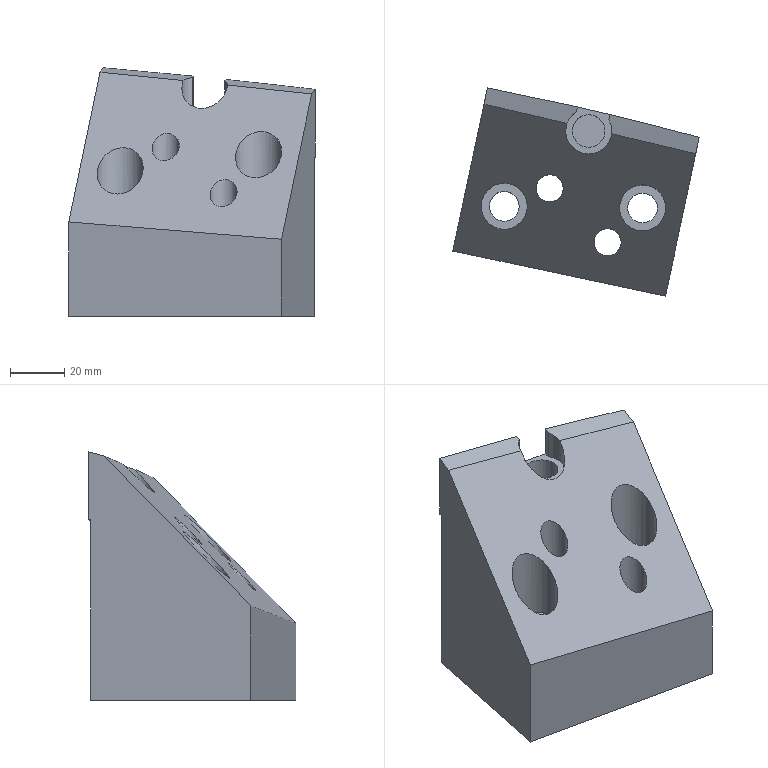Part | NX | features solid 2 | 1 solid | 24 faces | box 90.766 x 76.651 x 91.582 mm | volume 267587 mm3 | plane 11 | cylinder 8 | spline 5 | commonest cylinder face diameters 17 x3 10 x2 11 x2 12 x1
STEP:
#1=CARTESIAN_POINT('',(449.285,-481.788,-8.09));
#2=VERTEX_POINT('',#1);
#3=CARTESIAN_POINT('',(465.74,-485.634,-9.78));
#4=VERTEX_POINT('',#3);
#5=CARTESIAN_POINT('',(457.301,-484.613,-9.861));
#6=DIRECTION('',(-0.09165,-0.7023,0.706));
#7=DIRECTION('',(-0.09136,-0.7,-0.7082));
#8=AXIS2_PLACEMENT_3D('',#5,#6,#7);
#9=ELLIPSE('',#8,12.04,8.5);
#10=EDGE_CURVE('',#2,#4,#9,.T.);
#11=ORIENTED_EDGE('',*,*,#10,.F.);
#12=CARTESIAN_POINT('',(418.705,-474.755,-5.065));
#13=VERTEX_POINT('',#12);
#14=CARTESIAN_POINT('',(449.285,-481.788,-8.09));
#15=CARTESIAN_POINT('',(439.099,-479.42,-7.057));
#16=CARTESIAN_POINT('',(428.906,-477.075,-6.048));
#17=CARTESIAN_POINT('',(418.705,-474.755,-5.065));
#18=B_SPLINE_CURVE_WITH_KNOTS('',3,(#14,#15,#16,#17),.UNSPECIFIED.,.F.,.F.,(4,4),(0.,0.03152),.UNSPECIFIED.);
#19=EDGE_CURVE('',#2,#13,#18,.T.);
#20=ORIENTED_EDGE('',*,*,#19,.T.);
#21=CARTESIAN_POINT('',(407.237,-528.711,-60.225));
#22=VERTEX_POINT('',#21);
#23=CARTESIAN_POINT('',(413.497,-499.256,-30.113));
#24=DIRECTION('',(0.147,0.6917,0.7071));
#25=VECTOR('',#24,1000.);
#26=LINE('',#23,#25);
#27=EDGE_CURVE('',#13,#22,#26,.F.);
#28=ORIENTED_EDGE('',*,*,#27,.T.);
#29=CARTESIAN_POINT('',(485.592,-545.366,-66.621));
#30=VERTEX_POINT('',#29);
#31=CARTESIAN_POINT('',(402.563,-527.717,-59.844));
#32=DIRECTION('',(0.975,-0.2073,-0.07959));
#33=VECTOR('',#32,1000.);
#34=LINE('',#31,#33);
#35=EDGE_CURVE('',#22,#30,#34,.T.);
#36=ORIENTED_EDGE('',*,*,#35,.T.);
#37=CARTESIAN_POINT('',(496.726,-492.984,-13.069));
#38=VERTEX_POINT('',#37);
#39=CARTESIAN_POINT('',(492.518,-512.783,-33.311));
#40=DIRECTION('',(0.147,0.6917,0.7071));
#41=VECTOR('',#40,1000.);
#42=LINE('',#39,#41);
#43=EDGE_CURVE('',#30,#38,#42,.T.);
#44=ORIENTED_EDGE('',*,*,#43,.T.);
#45=CARTESIAN_POINT('',(496.726,-492.984,-13.069));
#46=CARTESIAN_POINT('',(486.404,-490.514,-11.952));
#47=CARTESIAN_POINT('',(476.076,-488.063,-10.855));
#48=CARTESIAN_POINT('',(465.74,-485.634,-9.78));
#49=B_SPLINE_CURVE_WITH_KNOTS('',3,(#45,#46,#47,#48),.UNSPECIFIED.,.F.,.F.,(4,4),(0.,0.03202),.UNSPECIFIED.);
#50=EDGE_CURVE('',#38,#4,#49,.T.);
#51=ORIENTED_EDGE('',*,*,#50,.T.);
#52=EDGE_LOOP('',(#11,#20,#28,#36,#44,#51));
#53=FACE_BOUND('',#52,.T.);
#54=CARTESIAN_POINT('',(464.904,-520.538,-44.609));
#55=VERTEX_POINT('',#54);
#56=CARTESIAN_POINT('',(464.257,-525.496,-49.625));
#57=DIRECTION('',(0.09165,0.7023,-0.706));
#58=DIRECTION('',(0.09136,0.7,0.7082));
#59=AXIS2_PLACEMENT_3D('',#56,#57,#58);
#60=ELLIPSE('',#59,7.082,5.);
#61=EDGE_CURVE('',#55,#55,#60,.F.);
#62=ORIENTED_EDGE('',*,*,#61,.F.);
#63=EDGE_LOOP('',(#62));
#64=FACE_BOUND('',#63,.T.);
#65=CARTESIAN_POINT('',(443.569,-500.668,-27.613));
#66=VERTEX_POINT('',#65);
#67=CARTESIAN_POINT('',(442.922,-505.626,-32.629));
#68=DIRECTION('',(0.09165,0.7023,-0.706));
#69=DIRECTION('',(0.09136,0.7,0.7082));
#70=AXIS2_PLACEMENT_3D('',#67,#68,#69);
#71=ELLIPSE('',#70,7.082,5.);
#72=EDGE_CURVE('',#66,#66,#71,.F.);
#73=ORIENTED_EDGE('',*,*,#72,.F.);
#74=EDGE_LOOP('',(#73));
#75=FACE_BOUND('',#74,.T.);
#76=CARTESIAN_POINT('',(478.257,-504.474,-26.897));
#77=VERTEX_POINT('',#76);
#78=CARTESIAN_POINT('',(477.158,-512.903,-35.424));
#79=DIRECTION('',(0.09165,0.7023,-0.706));
#80=DIRECTION('',(0.09136,0.7,0.7082));
#81=AXIS2_PLACEMENT_3D('',#78,#79,#80);
#82=ELLIPSE('',#81,12.04,8.5);
#83=EDGE_CURVE('',#77,#77,#82,.T.);
#84=ORIENTED_EDGE('',*,*,#83,.T.);
#85=EDGE_LOOP('',(#84));
#86=FACE_BOUND('',#85,.T.);
#87=CARTESIAN_POINT('',(427.271,-503.86,-32.905));
#88=VERTEX_POINT('',#87);
#89=CARTESIAN_POINT('',(426.171,-512.289,-41.432));
#90=DIRECTION('',(0.09165,0.7023,-0.706));
#91=DIRECTION('',(0.09136,0.7,0.7082));
#92=AXIS2_PLACEMENT_3D('',#89,#90,#91);
#93=ELLIPSE('',#92,12.04,8.5);
#94=EDGE_CURVE('',#88,#88,#93,.T.);
#95=ORIENTED_EDGE('',*,*,#94,.T.);
#96=EDGE_LOOP('',(#95));
#97=FACE_BOUND('',#96,.T.);
#98=CARTESIAN_POINT('',(496.103,-495.376,-15.53));
#99=DIRECTION('',(-0.09165,-0.7023,0.706));
#100=DIRECTION('',(0.,-0.709,-0.7052));
#101=AXIS2_PLACEMENT_3D('',#98,#99,#100);
#102=PLANE('',#101);
#103=ADVANCED_FACE('',(#53,#64,#75,#86,#97),#102,.T.);
#104=CARTESIAN_POINT('',(452.752,-477.433,-6.983));
#105=VERTEX_POINT('',#104);
#106=CARTESIAN_POINT('',(452.752,-477.433,-6.983));
#107=CARTESIAN_POINT('',(451.12,-478.467,-7.217));
#108=CARTESIAN_POINT('',(449.911,-480.01,-7.61));
#109=CARTESIAN_POINT('',(449.285,-481.788,-8.09));
#110=B_SPLINE_CURVE_WITH_KNOTS('',3,(#106,#107,#108,#109),.UNSPECIFIED.,.F.,.F.,(4,4),(0.,0.005753),.UNSPECIFIED.);
#111=EDGE_CURVE('',#105,#2,#110,.T.);
#112=ORIENTED_EDGE('',*,*,#111,.F.);
#113=CARTESIAN_POINT('',(453.112,-475.74,-6.517));
#114=VERTEX_POINT('',#113);
#115=CARTESIAN_POINT('',(452.752,-477.433,-6.983));
#116=CARTESIAN_POINT('',(452.872,-476.869,-6.827));
#117=CARTESIAN_POINT('',(452.992,-476.305,-6.672));
#118=CARTESIAN_POINT('',(453.112,-475.74,-6.517));
#119=B_SPLINE_CURVE_WITH_KNOTS('',3,(#115,#116,#117,#118),.UNSPECIFIED.,.F.,.F.,(4,4),(0.,0.001793),.UNSPECIFIED.);
#120=EDGE_CURVE('',#105,#114,#119,.T.);
#121=ORIENTED_EDGE('',*,*,#120,.T.);
#122=CARTESIAN_POINT('',(419.989,-468.715,-3.418));
#123=VERTEX_POINT('',#122);
#124=CARTESIAN_POINT('',(453.112,-475.74,-6.517));
#125=CARTESIAN_POINT('',(442.111,-473.238,-5.42));
#126=CARTESIAN_POINT('',(431.07,-470.895,-4.387));
#127=CARTESIAN_POINT('',(419.989,-468.715,-3.418));
#128=B_SPLINE_CURVE_WITH_KNOTS('',3,(#124,#125,#126,#127),.UNSPECIFIED.,.F.,.F.,(4,4),(0.,0.034),.UNSPECIFIED.);
#129=EDGE_CURVE('',#114,#123,#128,.T.);
#130=ORIENTED_EDGE('',*,*,#129,.T.);
#131=CARTESIAN_POINT('',(418.705,-474.755,-5.065));
#132=CARTESIAN_POINT('',(419.133,-472.742,-4.516));
#133=CARTESIAN_POINT('',(419.561,-470.729,-3.967));
#134=CARTESIAN_POINT('',(419.989,-468.715,-3.418));
#135=B_SPLINE_CURVE_WITH_KNOTS('',3,(#131,#132,#133,#134),.UNSPECIFIED.,.F.,.F.,(4,4),(0.,0.006391),.UNSPECIFIED.);
#136=EDGE_CURVE('',#13,#123,#135,.T.);
#137=ORIENTED_EDGE('',*,*,#136,.F.);
#138=ORIENTED_EDGE('',*,*,#19,.F.);
#139=EDGE_LOOP('',(#112,#121,#130,#137,#138));
#140=FACE_BOUND('',#139,.T.);
#141=CARTESIAN_POINT('',(419.708,-468.619,-3.382));
#142=CARTESIAN_POINT('',(418.384,-475.334,-5.216));
#143=CARTESIAN_POINT('',(430.965,-470.83,-4.365));
#144=CARTESIAN_POINT('',(429.58,-477.534,-6.199));
#145=CARTESIAN_POINT('',(442.182,-473.194,-5.41));
#146=CARTESIAN_POINT('',(440.732,-479.883,-7.244));
#147=CARTESIAN_POINT('',(453.348,-475.73,-6.522));
#148=CARTESIAN_POINT('',(451.829,-482.404,-8.356));
#149=B_SPLINE_SURFACE_WITH_KNOTS('',3,1,((#141,#142),(#143,#144),(#145,#146),(#147,#148)),.RULED_SURF.,.F.,.F.,.F.,(4,4),(2,2),(0.818,0.885),(0.2681,0.547),.PIECEWISE_BEZIER_KNOTS.);
#150=ADVANCED_FACE('',(#140),#149,.F.);
#151=CARTESIAN_POINT('',(464.757,-480.532,-8.293));
#152=VERTEX_POINT('',#151);
#153=CARTESIAN_POINT('',(465.74,-485.634,-9.78));
#154=CARTESIAN_POINT('',(465.953,-483.871,-9.287));
#155=CARTESIAN_POINT('',(465.612,-482.094,-8.768));
#156=CARTESIAN_POINT('',(464.757,-480.532,-8.293));
#157=B_SPLINE_CURVE_WITH_KNOTS('',3,(#153,#154,#155,#156),.UNSPECIFIED.,.F.,.F.,(4,4),(0.,0.00545),.UNSPECIFIED.);
#158=EDGE_CURVE('',#4,#152,#157,.T.);
#159=ORIENTED_EDGE('',*,*,#158,.F.);
#160=ORIENTED_EDGE('',*,*,#50,.F.);
#161=CARTESIAN_POINT('',(497.028,-491.564,-12.671));
#162=VERTEX_POINT('',#161);
#163=CARTESIAN_POINT('',(496.726,-492.984,-13.069));
#164=CARTESIAN_POINT('',(496.827,-492.511,-12.937));
#165=CARTESIAN_POINT('',(496.928,-492.037,-12.804));
#166=CARTESIAN_POINT('',(497.028,-491.564,-12.671));
#167=B_SPLINE_CURVE_WITH_KNOTS('',3,(#163,#164,#165,#166),.UNSPECIFIED.,.F.,.F.,(4,4),(0.009059,0.01057),.UNSPECIFIED.);
#168=EDGE_CURVE('',#38,#162,#167,.T.);
#169=ORIENTED_EDGE('',*,*,#168,.T.);
#170=CARTESIAN_POINT('',(498.002,-486.982,-11.386));
#171=VERTEX_POINT('',#170);
#172=CARTESIAN_POINT('',(497.028,-491.564,-12.671));
#173=CARTESIAN_POINT('',(497.353,-490.037,-12.243));
#174=CARTESIAN_POINT('',(497.678,-488.509,-11.814));
#175=CARTESIAN_POINT('',(498.002,-486.982,-11.386));
#176=B_SPLINE_CURVE_WITH_KNOTS('',3,(#172,#173,#174,#175),.UNSPECIFIED.,.F.,.F.,(4,4),(0.02436,0.02921),.UNSPECIFIED.);
#177=EDGE_CURVE('',#162,#171,#176,.T.);
#178=ORIENTED_EDGE('',*,*,#177,.T.);
#179=CARTESIAN_POINT('',(465.178,-478.555,-7.746));
#180=VERTEX_POINT('',#179);
#181=CARTESIAN_POINT('',(498.002,-486.982,-11.386));
#182=CARTESIAN_POINT('',(487.116,-483.988,-10.104));
#183=CARTESIAN_POINT('',(476.173,-481.185,-8.893));
#184=CARTESIAN_POINT('',(465.178,-478.555,-7.746));
#185=B_SPLINE_CURVE_WITH_KNOTS('',3,(#181,#182,#183,#184),.UNSPECIFIED.,.F.,.F.,(4,4),(0.,0.03408),.UNSPECIFIED.);
#186=EDGE_CURVE('',#171,#180,#185,.T.);
#187=ORIENTED_EDGE('',*,*,#186,.T.);
#188=CARTESIAN_POINT('',(465.178,-478.555,-7.746));
#189=CARTESIAN_POINT('',(465.038,-479.214,-7.929));
#190=CARTESIAN_POINT('',(464.898,-479.873,-8.111));
#191=CARTESIAN_POINT('',(464.757,-480.532,-8.293));
#192=B_SPLINE_CURVE_WITH_KNOTS('',3,(#188,#189,#190,#191),.UNSPECIFIED.,.F.,.F.,(4,4),(0.,0.002094),.UNSPECIFIED.);
#193=EDGE_CURVE('',#180,#152,#192,.T.);
#194=ORIENTED_EDGE('',*,*,#193,.T.);
#195=EDGE_LOOP('',(#159,#160,#169,#178,#187,#194));
#196=FACE_BOUND('',#195,.T.);
#197=CARTESIAN_POINT('',(464.991,-478.452,-7.71));
#198=CARTESIAN_POINT('',(463.397,-485.113,-9.546));
#199=CARTESIAN_POINT('',(476.244,-481.141,-8.882));
#200=CARTESIAN_POINT('',(474.577,-487.785,-10.718));
#201=CARTESIAN_POINT('',(487.44,-484.015,-10.124));
#202=CARTESIAN_POINT('',(485.695,-490.639,-11.96));
#203=CARTESIAN_POINT('',(498.568,-487.097,-11.441));
#204=CARTESIAN_POINT('',(496.741,-493.697,-13.276));
#205=B_SPLINE_SURFACE_WITH_KNOTS('',3,1,((#197,#198),(#199,#200),(#201,#202),(#203,#204)),.RULED_SURF.,.F.,.F.,.F.,(4,4),(2,2),(0.9084,0.9762),(0.2684,0.5476),.PIECEWISE_BEZIER_KNOTS.);
#206=ADVANCED_FACE('',(#196),#205,.F.);
#207=ORIENTED_EDGE('',*,*,#186,.F.);
#208=CARTESIAN_POINT('',(498.002,-486.982,-36.371));
#209=VERTEX_POINT('',#208);
#210=CARTESIAN_POINT('',(498.002,-486.982,-200.));
#211=DIRECTION('',(0.,0.,1.));
#212=VECTOR('',#211,1000.);
#213=LINE('',#210,#212);
#214=EDGE_CURVE('',#209,#171,#213,.T.);
#215=ORIENTED_EDGE('',*,*,#214,.F.);
#216=CARTESIAN_POINT('',(419.989,-468.715,-28.484));
#217=VERTEX_POINT('',#216);
#218=CARTESIAN_POINT('',(419.989,-468.715,-28.484));
#219=CARTESIAN_POINT('',(426.55,-470.006,-29.062));
#220=CARTESIAN_POINT('',(439.644,-472.702,-30.264));
#221=CARTESIAN_POINT('',(455.941,-476.352,-31.88));
#222=CARTESIAN_POINT('',(468.932,-479.444,-33.243));
#223=CARTESIAN_POINT('',(477.029,-481.453,-34.126));
#224=CARTESIAN_POINT('',(483.493,-483.107,-34.848));
#225=CARTESIAN_POINT('',(488.333,-484.372,-35.404));
#226=CARTESIAN_POINT('',(493.168,-485.661,-35.946));
#227=CARTESIAN_POINT('',(496.381,-486.536,-36.371));
#228=CARTESIAN_POINT('',(498.002,-486.982,-36.371));
#229=B_SPLINE_CURVE_WITH_KNOTS('',3,(#218,#219,#220,#221,#222,#223,#224,#225,#226,#227,#228),.UNSPECIFIED.,.F.,.F.,(4,1,1,1,1,1,1,1,4),(0.,0.02013,0.04027,0.05033,0.0604,0.06544,0.07047,0.0755,0.08054),.UNSPECIFIED.);
#230=EDGE_CURVE('',#217,#209,#229,.T.);
#231=ORIENTED_EDGE('',*,*,#230,.F.);
#232=CARTESIAN_POINT('',(419.989,-468.715,-200.));
#233=DIRECTION('',(0.,0.,1.));
#234=VECTOR('',#233,1000.);
#235=LINE('',#232,#234);
#236=EDGE_CURVE('',#217,#123,#235,.T.);
#237=ORIENTED_EDGE('',*,*,#236,.T.);
#238=ORIENTED_EDGE('',*,*,#129,.F.);
#239=CARTESIAN_POINT('',(453.112,-475.74,-19.));
#240=VERTEX_POINT('',#239);
#241=CARTESIAN_POINT('',(453.112,-475.74,-12.795));
#242=DIRECTION('',(0.,0.,1.));
#243=VECTOR('',#242,1000.);
#244=LINE('',#241,#243);
#245=EDGE_CURVE('',#240,#114,#244,.T.);
#246=ORIENTED_EDGE('',*,*,#245,.F.);
#247=CARTESIAN_POINT('',(465.178,-478.555,-19.));
#248=VERTEX_POINT('',#247);
#249=CARTESIAN_POINT('',(498.002,-486.982,-19.));
#250=CARTESIAN_POINT('',(487.75,-484.162,-19.));
#251=CARTESIAN_POINT('',(472.124,-480.143,-19.));
#252=CARTESIAN_POINT('',(446.106,-474.081,-19.));
#253=CARTESIAN_POINT('',(430.372,-470.758,-19.));
#254=CARTESIAN_POINT('',(419.989,-468.715,-19.));
#255=B_SPLINE_CURVE_WITH_KNOTS('',3,(#249,#250,#251,#252,#253,#254),.UNSPECIFIED.,.F.,.F.,(4,1,1,4),(0.,0.398,0.6039,1.),.UNSPECIFIED.);
#256=EDGE_CURVE('',#240,#248,#255,.F.);
#257=ORIENTED_EDGE('',*,*,#256,.T.);
#258=CARTESIAN_POINT('',(465.178,-478.555,-13.311));
#259=DIRECTION('',(0.,0.,1.));
#260=VECTOR('',#259,1000.);
#261=LINE('',#258,#260);
#262=EDGE_CURVE('',#180,#248,#261,.F.);
#263=ORIENTED_EDGE('',*,*,#262,.F.);
#264=EDGE_LOOP('',(#207,#215,#231,#237,#238,#246,#257,#263));
#265=FACE_BOUND('',#264,.T.);
#266=CARTESIAN_POINT('',(498.002,-486.982,-36.569));
#267=CARTESIAN_POINT('',(498.002,-486.982,-3.22));
#268=CARTESIAN_POINT('',(472.245,-479.897,-36.569));
#269=CARTESIAN_POINT('',(472.245,-479.897,-3.22));
#270=CARTESIAN_POINT('',(446.201,-473.872,-36.569));
#271=CARTESIAN_POINT('',(446.201,-473.872,-3.22));
#272=CARTESIAN_POINT('',(419.989,-468.715,-36.569));
#273=CARTESIAN_POINT('',(419.989,-468.715,-3.22));
#274=B_SPLINE_SURFACE_WITH_KNOTS('',3,1,((#266,#267),(#268,#269),(#270,#271),(#272,#273)),.SURF_OF_LINEAR_EXTRUSION.,.F.,.F.,.F.,(4,4),(2,2),(0.,1.),(0.,1.),.PIECEWISE_BEZIER_KNOTS.);
#275=ADVANCED_FACE('',(#265),#274,.T.);
#276=CARTESIAN_POINT('',(431.671,-512.289,-95.));
#277=VERTEX_POINT('',#276);
#278=CARTESIAN_POINT('',(426.171,-512.289,-95.));
#279=DIRECTION('',(0.,0.,1.));
#280=DIRECTION('',(1.,0.,0.));
#281=AXIS2_PLACEMENT_3D('',#278,#279,#280);
#282=CIRCLE('',#281,5.5);
#283=EDGE_CURVE('',#277,#277,#282,.T.);
#284=ORIENTED_EDGE('',*,*,#283,.T.);
#285=EDGE_LOOP('',(#284));
#286=FACE_BOUND('',#285,.T.);
#287=CARTESIAN_POINT('',(482.658,-512.903,-95.));
#288=VERTEX_POINT('',#287);
#289=CARTESIAN_POINT('',(477.158,-512.903,-95.));
#290=DIRECTION('',(0.,0.,1.));
#291=DIRECTION('',(1.,0.,0.));
#292=AXIS2_PLACEMENT_3D('',#289,#290,#291);
#293=CIRCLE('',#292,5.5);
#294=EDGE_CURVE('',#288,#288,#293,.T.);
#295=ORIENTED_EDGE('',*,*,#294,.T.);
#296=EDGE_LOOP('',(#295));
#297=FACE_BOUND('',#296,.T.);
#298=CARTESIAN_POINT('',(447.922,-505.626,-95.));
#299=VERTEX_POINT('',#298);
#300=CARTESIAN_POINT('',(442.922,-505.626,-95.));
#301=DIRECTION('',(0.,0.,1.));
#302=DIRECTION('',(1.,0.,0.));
#303=AXIS2_PLACEMENT_3D('',#300,#301,#302);
#304=CIRCLE('',#303,5.);
#305=EDGE_CURVE('',#299,#299,#304,.F.);
#306=ORIENTED_EDGE('',*,*,#305,.F.);
#307=EDGE_LOOP('',(#306));
#308=FACE_BOUND('',#307,.T.);
#309=CARTESIAN_POINT('',(419.781,-469.693,-95.));
#310=VERTEX_POINT('',#309);
#311=CARTESIAN_POINT('',(497.794,-487.962,-95.));
#312=VERTEX_POINT('',#311);
#313=CARTESIAN_POINT('',(419.781,-469.693,-95.));
#314=CARTESIAN_POINT('',(445.994,-474.85,-95.));
#315=CARTESIAN_POINT('',(472.036,-480.876,-95.));
#316=CARTESIAN_POINT('',(497.794,-487.962,-95.));
#317=B_SPLINE_CURVE_WITH_KNOTS('',3,(#313,#314,#315,#316),.UNSPECIFIED.,.F.,.F.,(4,4),(0.124,0.2041),.UNSPECIFIED.);
#318=EDGE_CURVE('',#310,#312,#317,.T.);
#319=ORIENTED_EDGE('',*,*,#318,.T.);
#320=CARTESIAN_POINT('',(485.592,-545.366,-95.));
#321=VERTEX_POINT('',#320);
#322=CARTESIAN_POINT('',(485.592,-545.366,-95.));
#323=DIRECTION('',(-0.2079,-0.9781,0.));
#324=VECTOR('',#323,1000.);
#325=LINE('',#322,#324);
#326=EDGE_CURVE('',#321,#312,#325,.F.);
#327=ORIENTED_EDGE('',*,*,#326,.F.);
#328=CARTESIAN_POINT('',(407.237,-528.711,-95.));
#329=VERTEX_POINT('',#328);
#330=CARTESIAN_POINT('',(407.237,-528.711,-95.));
#331=DIRECTION('',(-0.9781,0.2079,0.));
#332=VECTOR('',#331,1000.);
#333=LINE('',#330,#332);
#334=EDGE_CURVE('',#329,#321,#333,.F.);
#335=ORIENTED_EDGE('',*,*,#334,.F.);
#336=CARTESIAN_POINT('',(419.97,-468.803,-95.));
#337=DIRECTION('',(0.2079,0.9781,0.));
#338=VECTOR('',#337,1000.);
#339=LINE('',#336,#338);
#340=EDGE_CURVE('',#329,#310,#339,.T.);
#341=ORIENTED_EDGE('',*,*,#340,.T.);
#342=EDGE_LOOP('',(#319,#327,#335,#341));
#343=FACE_BOUND('',#342,.T.);
#344=CARTESIAN_POINT('',(469.257,-525.496,-95.));
#345=VERTEX_POINT('',#344);
#346=CARTESIAN_POINT('',(464.257,-525.496,-95.));
#347=DIRECTION('',(0.,0.,1.));
#348=DIRECTION('',(1.,0.,0.));
#349=AXIS2_PLACEMENT_3D('',#346,#347,#348);
#350=CIRCLE('',#349,5.);
#351=EDGE_CURVE('',#345,#345,#350,.F.);
#352=ORIENTED_EDGE('',*,*,#351,.F.);
#353=EDGE_LOOP('',(#352));
#354=FACE_BOUND('',#353,.T.);
#355=CARTESIAN_POINT('',(459.163,-477.134,-95.));
#356=DIRECTION('',(0.,0.,1.));
#357=DIRECTION('',(-1.,0.,0.));
#358=AXIS2_PLACEMENT_3D('',#355,#356,#357);
#359=PLANE('',#358);
#360=ADVANCED_FACE('',(#286,#297,#308,#343,#354),#359,.F.);
#361=CARTESIAN_POINT('',(407.237,-528.711,0.));
#362=DIRECTION('',(0.,0.,1.));
#363=VECTOR('',#362,1000.);
#364=LINE('',#361,#363);
#365=EDGE_CURVE('',#329,#22,#364,.T.);
#366=ORIENTED_EDGE('',*,*,#365,.F.);
#367=ORIENTED_EDGE('',*,*,#334,.T.);
#368=CARTESIAN_POINT('',(485.592,-545.366,0.));
#369=DIRECTION('',(0.,0.,1.));
#370=VECTOR('',#369,1000.);
#371=LINE('',#368,#370);
#372=EDGE_CURVE('',#321,#30,#371,.T.);
#373=ORIENTED_EDGE('',*,*,#372,.T.);
#374=ORIENTED_EDGE('',*,*,#35,.F.);
#375=EDGE_LOOP('',(#366,#367,#373,#374));
#376=FACE_BOUND('',#375,.T.);
#377=CARTESIAN_POINT('',(407.237,-528.711,0.));
#378=DIRECTION('',(-0.2079,-0.9781,0.));
#379=DIRECTION('',(0.9781,-0.2079,0.));
#380=AXIS2_PLACEMENT_3D('',#377,#378,#379);
#381=PLANE('',#380);
#382=ADVANCED_FACE('',(#376),#381,.T.);
#383=ORIENTED_EDGE('',*,*,#340,.F.);
#384=ORIENTED_EDGE('',*,*,#365,.T.);
#385=ORIENTED_EDGE('',*,*,#27,.F.);
#386=ORIENTED_EDGE('',*,*,#136,.T.);
#387=ORIENTED_EDGE('',*,*,#236,.F.);
#388=CARTESIAN_POINT('',(419.781,-469.693,-28.483));
#389=VERTEX_POINT('',#388);
#390=CARTESIAN_POINT('',(419.989,-468.715,-28.484));
#391=CARTESIAN_POINT('',(419.92,-469.041,-28.483));
#392=CARTESIAN_POINT('',(419.85,-469.367,-28.483));
#393=CARTESIAN_POINT('',(419.781,-469.693,-28.483));
#394=B_SPLINE_CURVE_WITH_KNOTS('',3,(#390,#391,#392,#393),.UNSPECIFIED.,.F.,.F.,(4,4),(0.,0.001),.UNSPECIFIED.);
#395=EDGE_CURVE('',#217,#389,#394,.T.);
#396=ORIENTED_EDGE('',*,*,#395,.T.);
#397=CARTESIAN_POINT('',(419.781,-469.693,-78.483));
#398=DIRECTION('',(0.,0.,-1.));
#399=VECTOR('',#398,1000.);
#400=LINE('',#397,#399);
#401=EDGE_CURVE('',#310,#389,#400,.F.);
#402=ORIENTED_EDGE('',*,*,#401,.F.);
#403=EDGE_LOOP('',(#383,#384,#385,#386,#387,#396,#402));
#404=FACE_BOUND('',#403,.T.);
#405=CARTESIAN_POINT('',(407.237,-528.711,0.));
#406=DIRECTION('',(0.9781,-0.2079,0.));
#407=DIRECTION('',(0.2079,0.9781,0.));
#408=AXIS2_PLACEMENT_3D('',#405,#406,#407);
#409=PLANE('',#408);
#410=ADVANCED_FACE('',(#404),#409,.F.);
#411=ORIENTED_EDGE('',*,*,#43,.F.);
#412=ORIENTED_EDGE('',*,*,#372,.F.);
#413=ORIENTED_EDGE('',*,*,#326,.T.);
#414=CARTESIAN_POINT('',(497.794,-487.962,-36.371));
#415=VERTEX_POINT('',#414);
#416=CARTESIAN_POINT('',(497.794,-487.962,-86.371));
#417=DIRECTION('',(0.,0.,-1.));
#418=VECTOR('',#417,1000.);
#419=LINE('',#416,#418);
#420=EDGE_CURVE('',#312,#415,#419,.F.);
#421=ORIENTED_EDGE('',*,*,#420,.T.);
#422=CARTESIAN_POINT('',(498.002,-486.982,-36.371));
#423=CARTESIAN_POINT('',(497.933,-487.309,-36.371));
#424=CARTESIAN_POINT('',(497.863,-487.635,-36.371));
#425=CARTESIAN_POINT('',(497.794,-487.962,-36.371));
#426=B_SPLINE_CURVE_WITH_KNOTS('',3,(#422,#423,#424,#425),.UNSPECIFIED.,.F.,.F.,(4,4),(0.,0.001002),.UNSPECIFIED.);
#427=EDGE_CURVE('',#209,#415,#426,.T.);
#428=ORIENTED_EDGE('',*,*,#427,.F.);
#429=ORIENTED_EDGE('',*,*,#214,.T.);
#430=ORIENTED_EDGE('',*,*,#177,.F.);
#431=ORIENTED_EDGE('',*,*,#168,.F.);
#432=EDGE_LOOP('',(#411,#412,#413,#421,#428,#429,#430,#431));
#433=FACE_BOUND('',#432,.T.);
#434=CARTESIAN_POINT('',(485.592,-545.366,0.));
#435=DIRECTION('',(0.9781,-0.2079,0.));
#436=DIRECTION('',(0.2079,0.9781,0.));
#437=AXIS2_PLACEMENT_3D('',#434,#435,#436);
#438=PLANE('',#437);
#439=ADVANCED_FACE('',(#433),#438,.T.);
#440=ORIENTED_EDGE('',*,*,#395,.F.);
#441=ORIENTED_EDGE('',*,*,#230,.T.);
#442=ORIENTED_EDGE('',*,*,#427,.T.);
#443=CARTESIAN_POINT('',(497.794,-487.962,-36.371));
#444=CARTESIAN_POINT('',(496.173,-487.516,-36.371));
#445=CARTESIAN_POINT('',(492.959,-486.641,-35.955));
#446=CARTESIAN_POINT('',(488.125,-485.35,-35.409));
#447=CARTESIAN_POINT('',(483.286,-484.085,-34.853));
#448=CARTESIAN_POINT('',(476.823,-482.428,-34.13));
#449=CARTESIAN_POINT('',(468.727,-480.416,-33.247));
#450=CARTESIAN_POINT('',(455.737,-477.32,-31.882));
#451=CARTESIAN_POINT('',(439.439,-473.674,-30.264));
#452=CARTESIAN_POINT('',(426.342,-470.984,-29.062));
#453=CARTESIAN_POINT('',(419.781,-469.693,-28.483));
#454=B_SPLINE_CURVE_WITH_KNOTS('',3,(#443,#444,#445,#446,#447,#448,#449,#450,#451,#452,#453),.UNSPECIFIED.,.F.,.F.,(4,1,1,1,1,1,1,1,4),(-0.0007328,0.06182,0.1244,0.1869,0.2495,0.3746,0.4997,0.75,1.),.UNSPECIFIED.);
#455=EDGE_CURVE('',#415,#389,#454,.T.);
#456=ORIENTED_EDGE('',*,*,#455,.T.);
#457=EDGE_LOOP('',(#440,#441,#442,#456));
#458=FACE_BOUND('',#457,.T.);
#459=CARTESIAN_POINT('',(498.528,-487.121,-36.371));
#460=CARTESIAN_POINT('',(498.353,-487.073,-36.371));
#461=CARTESIAN_POINT('',(498.179,-487.025,-36.371));
#462=CARTESIAN_POINT('',(498.004,-486.976,-36.371));
#463=CARTESIAN_POINT('',(496.383,-486.53,-36.371));
#464=CARTESIAN_POINT('',(494.776,-486.093,-36.149));
#465=CARTESIAN_POINT('',(491.557,-485.225,-35.775));
#466=CARTESIAN_POINT('',(489.946,-484.795,-35.587));
#467=CARTESIAN_POINT('',(485.109,-483.517,-35.031));
#468=CARTESIAN_POINT('',(481.88,-482.681,-34.666));
#469=CARTESIAN_POINT('',(472.178,-480.221,-33.59));
#470=CARTESIAN_POINT('',(465.691,-478.643,-32.897));
#471=CARTESIAN_POINT('',(446.182,-474.088,-30.887));
#472=CARTESIAN_POINT('',(433.111,-471.291,-29.641));
#473=CARTESIAN_POINT('',(419.99,-468.709,-28.484));
#474=CARTESIAN_POINT('',(419.828,-468.677,-28.47));
#475=CARTESIAN_POINT('',(419.665,-468.645,-28.455));
#476=CARTESIAN_POINT('',(419.502,-468.613,-28.441));
#477=CARTESIAN_POINT('',(498.261,-488.091,-36.371));
#478=CARTESIAN_POINT('',(498.086,-488.042,-36.371));
#479=CARTESIAN_POINT('',(497.912,-487.994,-36.371));
#480=CARTESIAN_POINT('',(497.737,-487.946,-36.371));
#481=CARTESIAN_POINT('',(496.117,-487.501,-36.371));
#482=CARTESIAN_POINT('',(494.513,-487.064,-36.149));
#483=CARTESIAN_POINT('',(491.296,-486.197,-35.775));
#484=CARTESIAN_POINT('',(489.687,-485.767,-35.587));
#485=CARTESIAN_POINT('',(484.855,-484.491,-35.031));
#486=CARTESIAN_POINT('',(481.629,-483.656,-34.666));
#487=CARTESIAN_POINT('',(471.937,-481.197,-33.59));
#488=CARTESIAN_POINT('',(465.456,-479.621,-32.897));
#489=CARTESIAN_POINT('',(445.966,-475.071,-30.887));
#490=CARTESIAN_POINT('',(432.906,-472.276,-29.641));
#491=CARTESIAN_POINT('',(419.796,-469.696,-28.484));
#492=CARTESIAN_POINT('',(419.634,-469.664,-28.47));
#493=CARTESIAN_POINT('',(419.471,-469.632,-28.455));
#494=CARTESIAN_POINT('',(419.309,-469.6,-28.441));
#495=B_SPLINE_SURFACE_WITH_KNOTS('',1,3,((#459,#460,#461,#462,#463,#464,#465,#466,#467,#468,#469,#470,#471,#472,#473,#474,#475,#476),(#477,#478,#479,#480,#481,#482,#483,#484,#485,#486,#487,#488,#489,#490,#491,#492,#493,#494)),.RULED_SURF.,.F.,.F.,.F.,(2,2),(4,3,2,2,2,2,3,4),(0.497,1.),(-0.006738,0.,0.0625,0.125,0.25,0.5,1.,1.006),.UNSPECIFIED.);
#496=ADVANCED_FACE('',(#458),#495,.T.);
#497=ORIENTED_EDGE('',*,*,#318,.F.);
#498=ORIENTED_EDGE('',*,*,#401,.T.);
#499=ORIENTED_EDGE('',*,*,#455,.F.);
#500=ORIENTED_EDGE('',*,*,#420,.F.);
#501=EDGE_LOOP('',(#497,#498,#499,#500));
#502=FACE_BOUND('',#501,.T.);
#503=CARTESIAN_POINT('',(497.794,-487.962,-36.371));
#504=CARTESIAN_POINT('',(497.794,-487.962,-103.287));
#505=CARTESIAN_POINT('',(496.175,-487.517,-36.371));
#506=CARTESIAN_POINT('',(496.175,-487.517,-103.287));
#507=CARTESIAN_POINT('',(492.958,-486.64,-35.955));
#508=CARTESIAN_POINT('',(492.958,-486.64,-102.872));
#509=CARTESIAN_POINT('',(488.126,-485.35,-35.409));
#510=CARTESIAN_POINT('',(488.126,-485.35,-102.326));
#511=CARTESIAN_POINT('',(483.286,-484.085,-34.853));
#512=CARTESIAN_POINT('',(483.286,-484.085,-101.769));
#513=CARTESIAN_POINT('',(476.823,-482.428,-34.13));
#514=CARTESIAN_POINT('',(476.823,-482.428,-101.046));
#515=CARTESIAN_POINT('',(468.726,-480.416,-33.247));
#516=CARTESIAN_POINT('',(468.726,-480.416,-100.163));
#517=CARTESIAN_POINT('',(455.738,-477.32,-31.882));
#518=CARTESIAN_POINT('',(455.738,-477.32,-98.799));
#519=CARTESIAN_POINT('',(439.437,-473.673,-30.264));
#520=CARTESIAN_POINT('',(439.437,-473.673,-97.181));
#521=CARTESIAN_POINT('',(426.348,-470.985,-29.062));
#522=CARTESIAN_POINT('',(426.348,-470.985,-95.978));
#523=CARTESIAN_POINT('',(419.781,-469.693,-28.483));
#524=CARTESIAN_POINT('',(419.781,-469.693,-95.399));
#525=B_SPLINE_SURFACE_WITH_KNOTS('',3,1,((#503,#504),(#505,#506),(#507,#508),(#509,#510),(#511,#512),(#513,#514),(#515,#516),(#517,#518),(#519,#520),(#521,#522),(#523,#524)),.SURF_OF_LINEAR_EXTRUSION.,.F.,.F.,.F.,(4,1,1,1,1,1,1,1,4),(2,2),(-0.0007336,0.06182,0.1244,0.1869,0.2495,0.3746,0.4997,0.75,1.),(0.,1.),.UNSPECIFIED.);
#526=ADVANCED_FACE('',(#502),#525,.F.);
#527=ORIENTED_EDGE('',*,*,#305,.T.);
#528=EDGE_LOOP('',(#527));
#529=FACE_BOUND('',#528,.T.);
#530=ORIENTED_EDGE('',*,*,#72,.T.);
#531=EDGE_LOOP('',(#530));
#532=FACE_BOUND('',#531,.T.);
#533=CARTESIAN_POINT('',(442.922,-505.626,-200.));
#534=DIRECTION('',(0.,0.,1.));
#535=DIRECTION('',(-1.,0.,0.));
#536=AXIS2_PLACEMENT_3D('',#533,#534,#535);
#537=CYLINDRICAL_SURFACE('',#536,5.);
#538=ADVANCED_FACE('',(#529,#532),#537,.F.);
#539=ORIENTED_EDGE('',*,*,#351,.T.);
#540=EDGE_LOOP('',(#539));
#541=FACE_BOUND('',#540,.T.);
#542=ORIENTED_EDGE('',*,*,#61,.T.);
#543=EDGE_LOOP('',(#542));
#544=FACE_BOUND('',#543,.T.);
#545=CARTESIAN_POINT('',(464.257,-525.496,-200.));
#546=DIRECTION('',(0.,0.,1.));
#547=DIRECTION('',(-1.,0.,0.));
#548=AXIS2_PLACEMENT_3D('',#545,#546,#547);
#549=CYLINDRICAL_SURFACE('',#548,5.);
#550=ADVANCED_FACE('',(#541,#544),#549,.F.);
#551=ORIENTED_EDGE('',*,*,#294,.F.);
#552=EDGE_LOOP('',(#551));
#553=FACE_BOUND('',#552,.T.);
#554=CARTESIAN_POINT('',(482.658,-512.903,-60.));
#555=VERTEX_POINT('',#554);
#556=CARTESIAN_POINT('',(477.158,-512.903,-60.));
#557=DIRECTION('',(0.,0.,1.));
#558=DIRECTION('',(1.,0.,0.));
#559=AXIS2_PLACEMENT_3D('',#556,#557,#558);
#560=CIRCLE('',#559,5.5);
#561=EDGE_CURVE('',#555,#555,#560,.F.);
#562=ORIENTED_EDGE('',*,*,#561,.F.);
#563=EDGE_LOOP('',(#562));
#564=FACE_BOUND('',#563,.T.);
#565=CARTESIAN_POINT('',(477.158,-512.903,-105.));
#566=DIRECTION('',(0.,0.,1.));
#567=DIRECTION('',(-1.,0.,0.));
#568=AXIS2_PLACEMENT_3D('',#565,#566,#567);
#569=CYLINDRICAL_SURFACE('',#568,5.5);
#570=ADVANCED_FACE('',(#553,#564),#569,.F.);
#571=ORIENTED_EDGE('',*,*,#561,.T.);
#572=EDGE_LOOP('',(#571));
#573=FACE_BOUND('',#572,.T.);
#574=CARTESIAN_POINT('',(485.658,-512.903,-60.));
#575=VERTEX_POINT('',#574);
#576=CARTESIAN_POINT('',(477.158,-512.903,-60.));
#577=DIRECTION('',(0.,0.,1.));
#578=DIRECTION('',(1.,0.,0.));
#579=AXIS2_PLACEMENT_3D('',#576,#577,#578);
#580=CIRCLE('',#579,8.5);
#581=EDGE_CURVE('',#575,#575,#580,.F.);
#582=ORIENTED_EDGE('',*,*,#581,.F.);
#583=EDGE_LOOP('',(#582));
#584=FACE_BOUND('',#583,.T.);
#585=CARTESIAN_POINT('',(477.158,-512.903,-60.));
#586=DIRECTION('',(0.,0.,-1.));
#587=DIRECTION('',(1.,0.,0.));
#588=AXIS2_PLACEMENT_3D('',#585,#586,#587);
#589=PLANE('',#588);
#590=ADVANCED_FACE('',(#573,#584),#589,.F.);
#591=ORIENTED_EDGE('',*,*,#83,.F.);
#592=EDGE_LOOP('',(#591));
#593=FACE_BOUND('',#592,.T.);
#594=ORIENTED_EDGE('',*,*,#581,.T.);
#595=EDGE_LOOP('',(#594));
#596=FACE_BOUND('',#595,.T.);
#597=CARTESIAN_POINT('',(477.158,-512.903,-65.));
#598=DIRECTION('',(0.,0.,1.));
#599=DIRECTION('',(-1.,0.,0.));
#600=AXIS2_PLACEMENT_3D('',#597,#598,#599);
#601=CYLINDRICAL_SURFACE('',#600,8.5);
#602=ADVANCED_FACE('',(#593,#596),#601,.F.);
#603=ORIENTED_EDGE('',*,*,#283,.F.);
#604=EDGE_LOOP('',(#603));
#605=FACE_BOUND('',#604,.T.);
#606=CARTESIAN_POINT('',(431.671,-512.289,-60.));
#607=VERTEX_POINT('',#606);
#608=CARTESIAN_POINT('',(426.171,-512.289,-60.));
#609=DIRECTION('',(0.,0.,1.));
#610=DIRECTION('',(1.,0.,0.));
#611=AXIS2_PLACEMENT_3D('',#608,#609,#610);
#612=CIRCLE('',#611,5.5);
#613=EDGE_CURVE('',#607,#607,#612,.F.);
#614=ORIENTED_EDGE('',*,*,#613,.F.);
#615=EDGE_LOOP('',(#614));
#616=FACE_BOUND('',#615,.T.);
#617=CARTESIAN_POINT('',(426.171,-512.289,-105.));
#618=DIRECTION('',(0.,0.,1.));
#619=DIRECTION('',(-1.,0.,0.));
#620=AXIS2_PLACEMENT_3D('',#617,#618,#619);
#621=CYLINDRICAL_SURFACE('',#620,5.5);
#622=ADVANCED_FACE('',(#605,#616),#621,.F.);
#623=ORIENTED_EDGE('',*,*,#613,.T.);
#624=EDGE_LOOP('',(#623));
#625=FACE_BOUND('',#624,.T.);
#626=CARTESIAN_POINT('',(434.671,-512.289,-60.));
#627=VERTEX_POINT('',#626);
#628=CARTESIAN_POINT('',(426.171,-512.289,-60.));
#629=DIRECTION('',(0.,0.,1.));
#630=DIRECTION('',(1.,0.,0.));
#631=AXIS2_PLACEMENT_3D('',#628,#629,#630);
#632=CIRCLE('',#631,8.5);
#633=EDGE_CURVE('',#627,#627,#632,.F.);
#634=ORIENTED_EDGE('',*,*,#633,.F.);
#635=EDGE_LOOP('',(#634));
#636=FACE_BOUND('',#635,.T.);
#637=CARTESIAN_POINT('',(426.171,-512.289,-60.));
#638=DIRECTION('',(0.,0.,-1.));
#639=DIRECTION('',(1.,0.,0.));
#640=AXIS2_PLACEMENT_3D('',#637,#638,#639);
#641=PLANE('',#640);
#642=ADVANCED_FACE('',(#625,#636),#641,.F.);
#643=ORIENTED_EDGE('',*,*,#94,.F.);
#644=EDGE_LOOP('',(#643));
#645=FACE_BOUND('',#644,.T.);
#646=ORIENTED_EDGE('',*,*,#633,.T.);
#647=EDGE_LOOP('',(#646));
#648=FACE_BOUND('',#647,.T.);
#649=CARTESIAN_POINT('',(426.171,-512.289,-65.));
#650=DIRECTION('',(0.,0.,1.));
#651=DIRECTION('',(-1.,0.,0.));
#652=AXIS2_PLACEMENT_3D('',#649,#650,#651);
#653=CYLINDRICAL_SURFACE('',#652,8.5);
#654=ADVANCED_FACE('',(#645,#648),#653,.F.);
#655=CARTESIAN_POINT('',(463.301,-484.613,-19.));
#656=VERTEX_POINT('',#655);
#657=CARTESIAN_POINT('',(457.301,-484.613,-19.));
#658=DIRECTION('',(0.,0.,1.));
#659=DIRECTION('',(1.,0.,0.));
#660=AXIS2_PLACEMENT_3D('',#657,#658,#659);
#661=CIRCLE('',#660,6.);
#662=EDGE_CURVE('',#656,#656,#661,.T.);
#663=ORIENTED_EDGE('',*,*,#662,.F.);
#664=EDGE_LOOP('',(#663));
#665=FACE_BOUND('',#664,.T.);
#666=CARTESIAN_POINT('',(452.752,-477.433,-19.));
#667=VERTEX_POINT('',#666);
#668=CARTESIAN_POINT('',(451.465,-483.489,-19.));
#669=DIRECTION('',(0.2079,0.9781,0.));
#670=VECTOR('',#669,1000.);
#671=LINE('',#668,#670);
#672=EDGE_CURVE('',#240,#667,#671,.F.);
#673=ORIENTED_EDGE('',*,*,#672,.T.);
#674=CARTESIAN_POINT('',(464.757,-480.532,-19.));
#675=VERTEX_POINT('',#674);
#676=CARTESIAN_POINT('',(457.301,-484.613,-19.));
#677=DIRECTION('',(0.,0.,-1.));
#678=DIRECTION('',(-1.,0.,0.));
#679=AXIS2_PLACEMENT_3D('',#676,#677,#678);
#680=CIRCLE('',#679,8.5);
#681=EDGE_CURVE('',#675,#667,#680,.T.);
#682=ORIENTED_EDGE('',*,*,#681,.F.);
#683=CARTESIAN_POINT('',(465.202,-478.442,-19.));
#684=DIRECTION('',(0.2079,0.9781,0.));
#685=VECTOR('',#684,1000.);
#686=LINE('',#683,#685);
#687=EDGE_CURVE('',#248,#675,#686,.F.);
#688=ORIENTED_EDGE('',*,*,#687,.F.);
#689=ORIENTED_EDGE('',*,*,#256,.F.);
#690=EDGE_LOOP('',(#673,#682,#688,#689));
#691=FACE_BOUND('',#690,.T.);
#692=CARTESIAN_POINT('',(457.177,-484.703,-19.));
#693=DIRECTION('',(0.,0.,1.));
#694=DIRECTION('',(-1.,0.,0.));
#695=AXIS2_PLACEMENT_3D('',#692,#693,#694);
#696=PLANE('',#695);
#697=ADVANCED_FACE('',(#665,#691),#696,.T.);
#698=ORIENTED_EDGE('',*,*,#120,.F.);
#699=CARTESIAN_POINT('',(452.752,-477.433,-6.958));
#700=DIRECTION('',(0.,0.,-1.));
#701=VECTOR('',#700,1000.);
#702=LINE('',#699,#701);
#703=EDGE_CURVE('',#105,#667,#702,.T.);
#704=ORIENTED_EDGE('',*,*,#703,.T.);
#705=ORIENTED_EDGE('',*,*,#672,.F.);
#706=ORIENTED_EDGE('',*,*,#245,.T.);
#707=EDGE_LOOP('',(#698,#704,#705,#706));
#708=FACE_BOUND('',#707,.T.);
#709=CARTESIAN_POINT('',(453.085,-475.866,-19.));
#710=DIRECTION('',(0.9781,-0.2079,0.));
#711=DIRECTION('',(0.,0.,1.));
#712=AXIS2_PLACEMENT_3D('',#709,#710,#711);
#713=PLANE('',#712);
#714=ADVANCED_FACE('',(#708),#713,.T.);
#715=ORIENTED_EDGE('',*,*,#687,.T.);
#716=CARTESIAN_POINT('',(464.757,-480.532,-19.));
#717=DIRECTION('',(0.,0.,-1.));
#718=VECTOR('',#717,1000.);
#719=LINE('',#716,#718);
#720=EDGE_CURVE('',#675,#152,#719,.F.);
#721=ORIENTED_EDGE('',*,*,#720,.T.);
#722=ORIENTED_EDGE('',*,*,#193,.F.);
#723=ORIENTED_EDGE('',*,*,#262,.T.);
#724=EDGE_LOOP('',(#715,#721,#722,#723));
#725=FACE_BOUND('',#724,.T.);
#726=CARTESIAN_POINT('',(465.202,-478.442,-19.));
#727=DIRECTION('',(-0.9781,0.2079,0.));
#728=DIRECTION('',(0.,0.,1.));
#729=AXIS2_PLACEMENT_3D('',#726,#727,#728);
#730=PLANE('',#729);
#731=ADVANCED_FACE('',(#725),#730,.T.);
#732=ORIENTED_EDGE('',*,*,#111,.T.);
#733=ORIENTED_EDGE('',*,*,#10,.T.);
#734=ORIENTED_EDGE('',*,*,#158,.T.);
#735=ORIENTED_EDGE('',*,*,#720,.F.);
#736=ORIENTED_EDGE('',*,*,#681,.T.);
#737=ORIENTED_EDGE('',*,*,#703,.F.);
#738=EDGE_LOOP('',(#732,#733,#734,#735,#736,#737));
#739=FACE_BOUND('',#738,.T.);
#740=CARTESIAN_POINT('',(457.301,-484.613,81.));
#741=DIRECTION('',(0.,0.,-1.));
#742=DIRECTION('',(-1.,0.,0.));
#743=AXIS2_PLACEMENT_3D('',#740,#741,#742);
#744=CYLINDRICAL_SURFACE('',#743,8.5);
#745=ADVANCED_FACE('',(#739),#744,.F.);
#746=ORIENTED_EDGE('',*,*,#662,.T.);
#747=EDGE_LOOP('',(#746));
#748=FACE_BOUND('',#747,.T.);
#749=CARTESIAN_POINT('',(451.301,-484.613,-44.));
#750=VERTEX_POINT('',#749);
#751=CARTESIAN_POINT('',(457.301,-484.613,-44.));
#752=DIRECTION('',(0.,0.,-1.));
#753=DIRECTION('',(-1.,0.,0.));
#754=AXIS2_PLACEMENT_3D('',#751,#752,#753);
#755=CIRCLE('',#754,6.);
#756=EDGE_CURVE('',#750,#750,#755,.T.);
#757=ORIENTED_EDGE('',*,*,#756,.T.);
#758=EDGE_LOOP('',(#757));
#759=FACE_BOUND('',#758,.T.);
#760=CARTESIAN_POINT('',(457.301,-484.613,66.));
#761=DIRECTION('',(0.,0.,-1.));
#762=DIRECTION('',(-1.,0.,0.));
#763=AXIS2_PLACEMENT_3D('',#760,#761,#762);
#764=CYLINDRICAL_SURFACE('',#763,6.);
#765=ADVANCED_FACE('',(#748,#759),#764,.F.);
#766=ORIENTED_EDGE('',*,*,#756,.F.);
#767=EDGE_LOOP('',(#766));
#768=FACE_BOUND('',#767,.T.);
#769=CARTESIAN_POINT('',(457.177,-484.703,-44.));
#770=DIRECTION('',(0.,0.,1.));
#771=DIRECTION('',(-1.,0.,0.));
#772=AXIS2_PLACEMENT_3D('',#769,#770,#771);
#773=PLANE('',#772);
#774=ADVANCED_FACE('',(#768),#773,.T.);
#775=CLOSED_SHELL('',(#103,#150,#206,#275,#360,#382,#410,#439,#496,#526,#538,#550,#570,#590,#602,#622,#642,#654,#697,#714,#731,#745,#765,#774));
#776=MANIFOLD_SOLID_BREP('',#775);
#777=(LENGTH_UNIT()NAMED_UNIT(*)SI_UNIT(.MILLI.,.METRE.));
#778=UNCERTAINTY_MEASURE_WITH_UNIT(LENGTH_MEASURE(0.0508),#777,'','');
#779=(NAMED_UNIT(*)PLANE_ANGLE_UNIT()SI_UNIT($,.RADIAN.));
#780=(NAMED_UNIT(*)SI_UNIT($,.STERADIAN.)SOLID_ANGLE_UNIT());
#781=(GEOMETRIC_REPRESENTATION_CONTEXT(3)GLOBAL_UNCERTAINTY_ASSIGNED_CONTEXT((#778))GLOBAL_UNIT_ASSIGNED_CONTEXT((#777,#779,#780))REPRESENTATION_CONTEXT('',''));
#782=ADVANCED_BREP_SHAPE_REPRESENTATION('',(#776),#781);